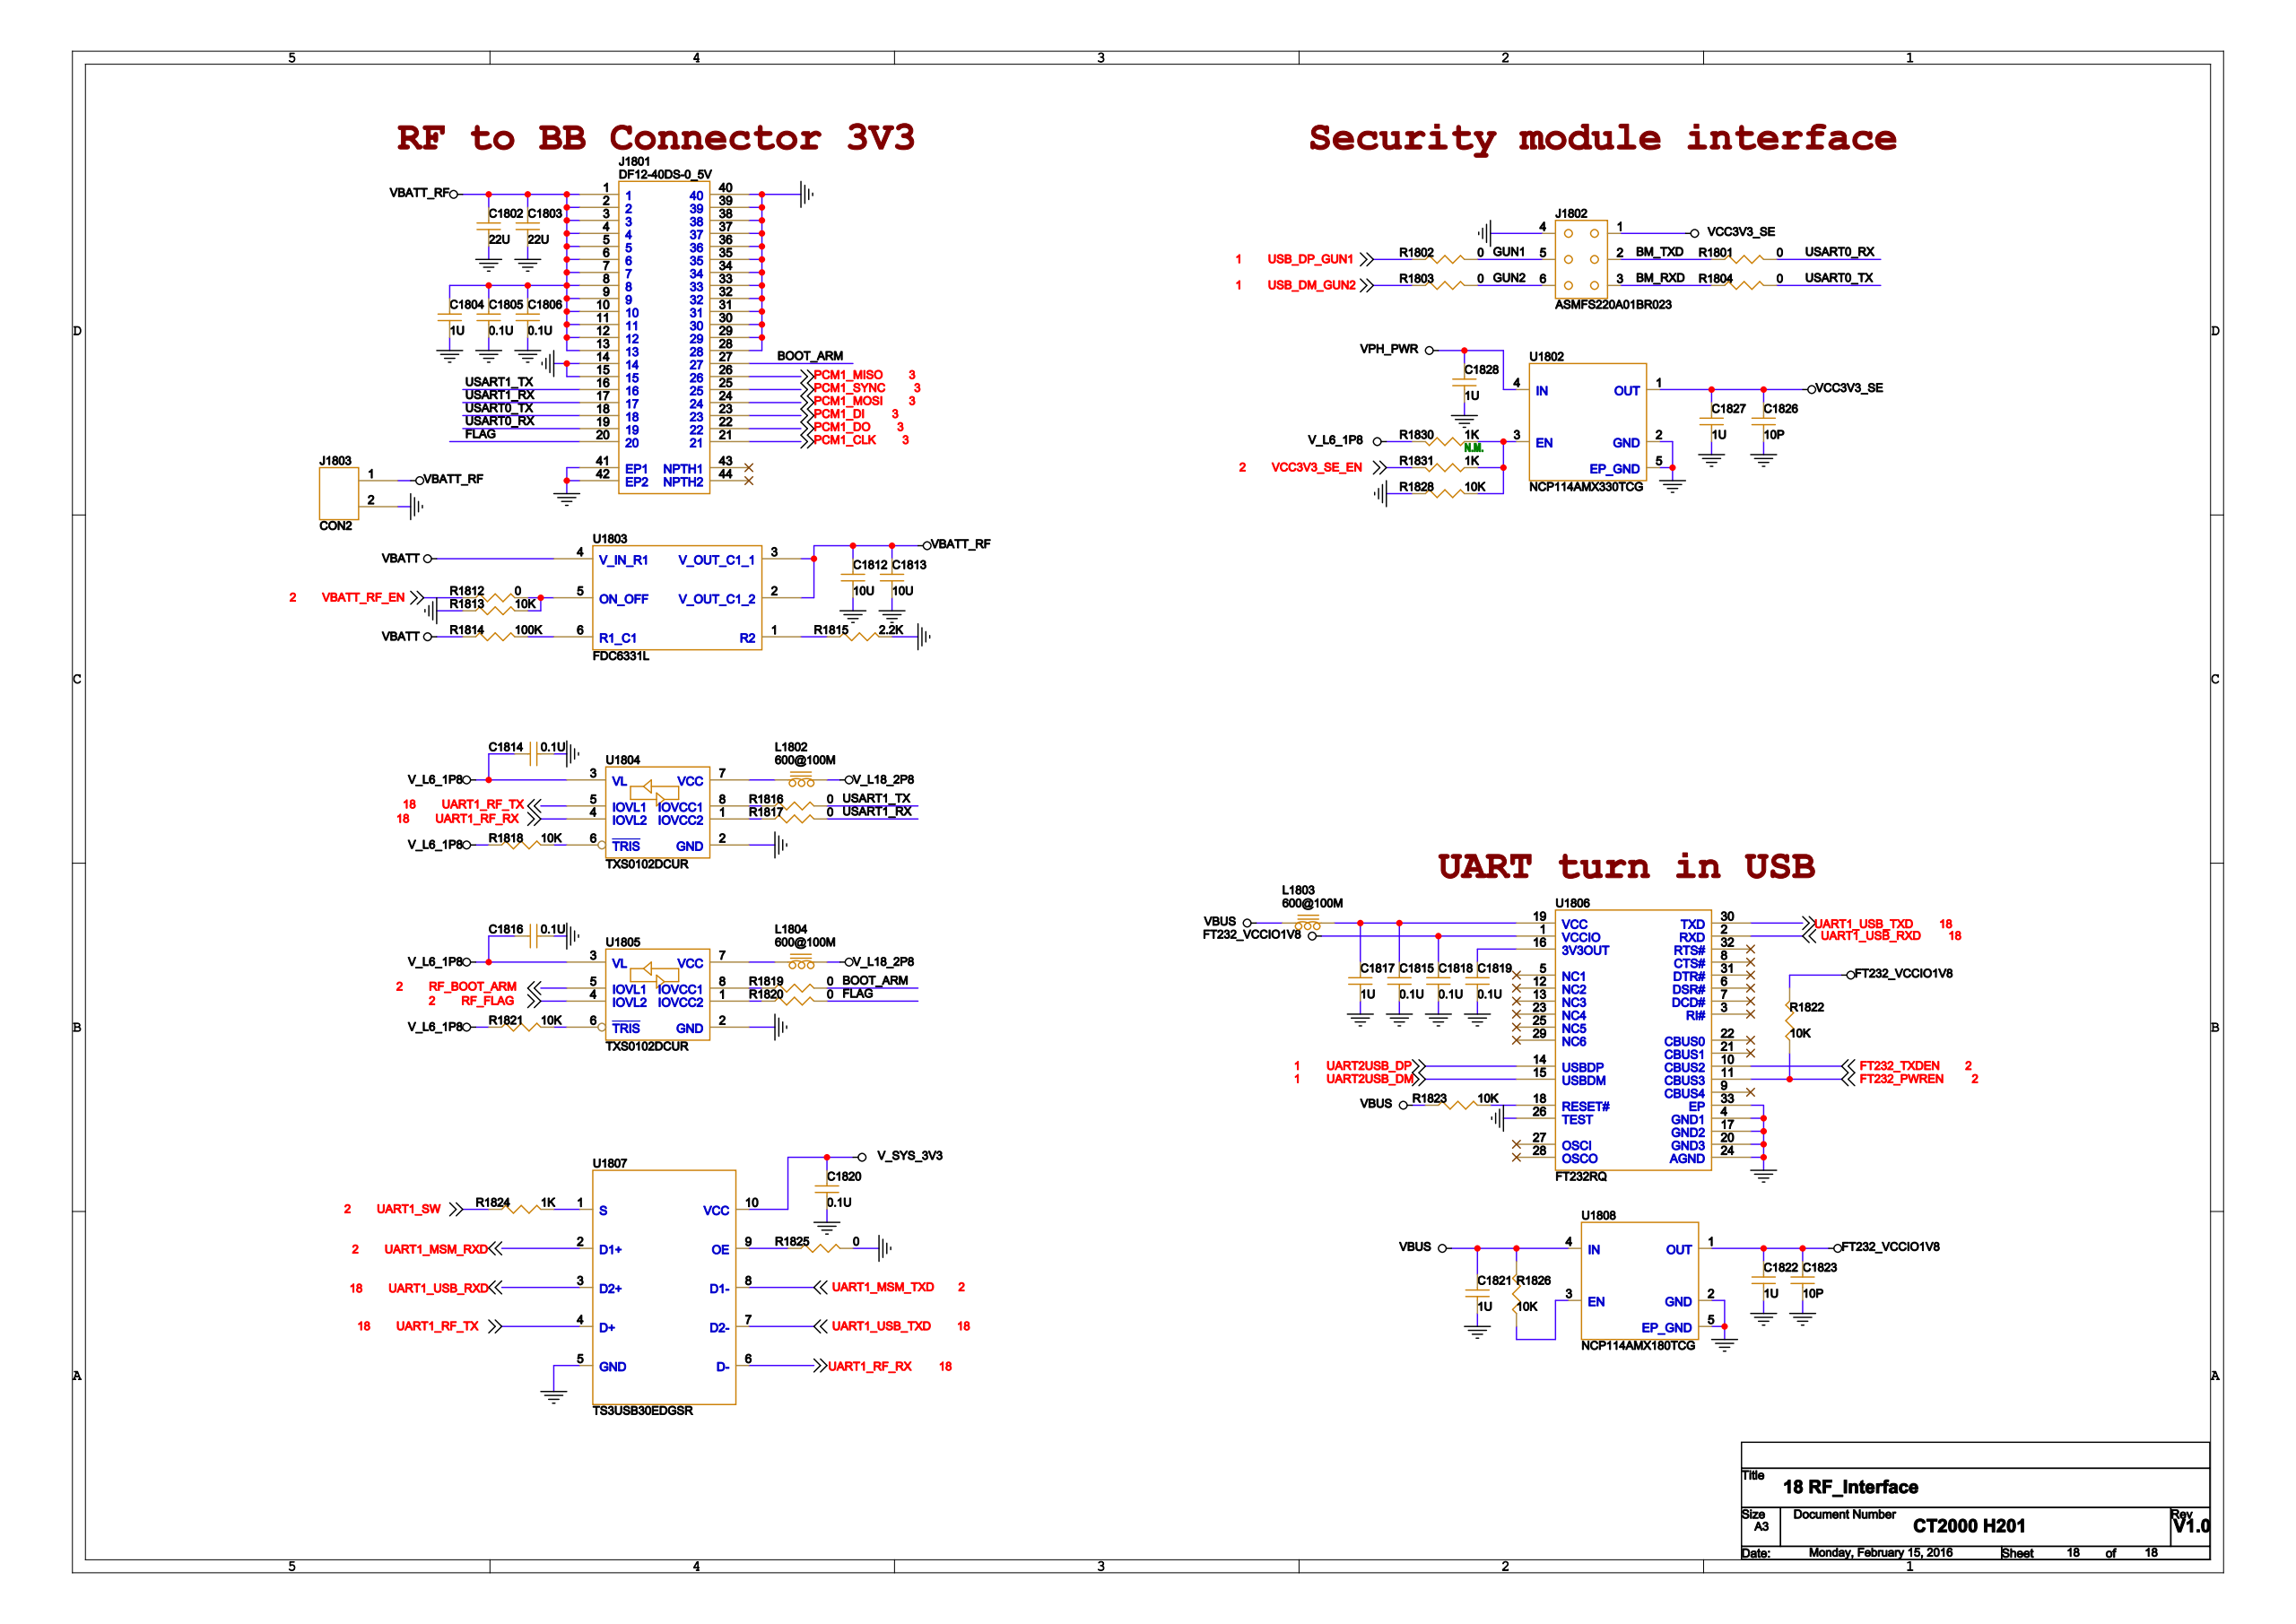Circuit board | Cadence Allegro | 573 parts | 376 nets | one sheet of the schematic
Parts on this sheet (reference | value | footprint):
C1802 | 22U | C0805
C1803 | 22U | C0805
C1804 | 1U | C0402
C1805 | 0.1U | C0402
C1806 | 0.1U | C0402
C1812 | 10U | C0603
C1813 | 10U | C0603
C1814 | 0.1U | C0402
C1815 | 0.1U | C0402
C1816 | 0.1U | C0402
C1817 | 1U | C0402
C1818 | 0.1U | C0402
C1819 | 0.1U | C0402
C1820 | 0.1U | C0402
C1821 | 1U | C0402
C1822 | 1U | C0402
C1823 | 10P | C0402
C1826 | 10P | C0402
C1827 | 1U | C0402
C1828 | 1U | C0402
J1801 | DF12-40DS-0_5V | BTB_DF12-40DS-0_5V_CCW
J1802 | ASMFS220A01BR023 | CON6_ASMFS220A01BR023
J1803 | CON2 | SIP2_2_54P
L1802 | 600@100M | L0402
L1803 | 600@100M | L0402
L1804 | 600@100M | L0402
R1801 | 0 | R0402
R1802 | 0 | R0402
R1803 | 0 | R0402
R1804 | 0 | R0402
R1812 | 0 | R0402
R1813 | 10K | R0402
R1814 | 100K | R0402
R1815 | 2.2K | R0402
R1816 | 0 | R0402
R1817 | 0 | R0402
R1818 | 10K | R0402
R1819 | 0 | R0402
R1820 | 0 | R0402
R1821 | 10K | R0402
R1822 | 10K | R0402
R1823 | 10K | R0402
R1824 | 1K | R0402
R1825 | 0 | R0402
R1826 | 10K | R0402
R1828 | 10K | R0402
R1830 | 1K | R0402
R1831 | 1K | R0402
U1802 | NCP114AMX330TCG | UDFN4_1X1X0P7_0P65
U1803 | FDC6331L | SSOT6_1P7X3
U1804 | TXS0102DCUR | SOT-70
U1805 | TXS0102DCUR | SOT-70
U1806 | FT232RQ | QFN32_5X5X0P9_0P5
U1807 | TS3USB30EDGSR | TS3USB30EDGSR
U1808 | NCP114AMX180TCG | UDFN4_1X1X0P7_0P65
Nets of these parts (net: part-pin ...):
GND: C1802-2 C1803-2 C1804-2 C1805-2 C1806-2 C1812-2 C1813-2 C1814-2 C1815-2 C1816-2 C1817-2 C1818-2 C1819-2 C1820-2 C1821-2 C1822-2 C1823-2 C1826-2 C1827-2 C1828-2 J1802-4 J1803-2 R1813-2 R1815-2 R1825-2 R1828-1 U1802-2 U1802-5 U1804-2 U1805-2 U1806-4 U1806-17 U1806-20 U1806-24 U1806-26 U1806-33 U1807-5 U1808-2 U1808-5 J1801-1 J1801-2 J1801-3 J1801-4 J1801-5 J1801-6 J1801-7 J1801-8 J1801-9 J1801-10 J1801-11 J1801-12 J1801-13 J1801-26 J1801-27 J1801-41 J1801-42
N52696315: C1819-1 U1806-16
FT232_TXDEN: U1806-10
FT232_PWREN: R1822-2 U1806-11
N52696194: R1823-1 U1806-18
UART1_USB_RXD: U1806-2 U1807-3
UART1_USB_TXD: U1806-30 U1807-7
UART2USB_DM: U1806-15
UART2USB_DP: U1806-14
N52698432: C1815-1 C1817-1 L1803-1 U1806-19
FT232_VCCIO1V8: C1818-1 C1822-1 C1823-1 R1822-1 U1806-1 U1808-1
V_SYS_3V3: C1820-1 U1807-10
VBATT: R1814-1 U1803-4
VPH_PWR: C1828-1 U1802-4
BOOT_ARM: R1819-2 J1801-14
PCM1_MISO: J1801-15
PCM1_SYNC: J1801-16
PCM1_MOSI: J1801-17
PCM1_DI: J1801-18
PCM1_DO: J1801-19
PCM1_CLK: J1801-20
FLAG: R1820-2 J1801-21
USART0_RX: R1801-2 J1801-22
USART0_TX: R1804-2 J1801-23
USART1_RX: R1817-2 J1801-24
USART1_TX: R1816-2 J1801-25
VBATT_RF: C1802-1 C1803-1 C1804-1 C1805-1 C1806-1 C1812-1 C1813-1 J1803-1 U1803-2 U1803-3 J1801-28 J1801-29 J1801-30 J1801-31 J1801-32 J1801-33 J1801-34 J1801-35 J1801-36 J1801-37 J1801-38 J1801-39 J1801-40
VCC3V3_SE: C1826-1 C1827-1 J1802-1 U1802-1
BM_TXD: J1802-2 R1801-1
BM_RXD: J1802-3 R1804-1
GUN1: J1802-5 R1802-2
GUN2: J1802-6 R1803-2
USB_DM_GUN2: R1803-1
USB_DP_GUN1: R1802-1
N52704005: R1826-2 U1808-3
VBUS: C1821-1 L1803-2 R1823-2 R1826-1 U1808-4
VBATT_RF_EN: R1812-1
UART1_MSM_RXD: U1807-2
UART1_MSM_TXD: U1807-8
V_L6_1P8: C1814-1 C1816-1 R1818-1 R1821-1 R1830-2 U1804-3 U1805-3
RF_BOOT_ARM: U1805-5
RF_FLAG: U1805-4
VCC3V3_SE_EN: R1831-2
UART1_SW: R1824-1
VCC3V3_RFIO: L1802-2 L1804-2
N52755623: L1802-1 U1804-7
N52758844: L1804-1 U1805-7
N52856260: R1828-2 R1830-1 R1831-1 U1802-3
N52674574: R1812-2 R1813-1 U1803-5
N52755629: R1818-2 U1804-6
N52758850: R1821-2 U1805-6
N52757691: R1816-1 U1804-8
N52755610: R1817-1 U1804-1
N52758889: R1819-1 U1805-8
N52758830: R1820-1 U1805-1
N52583772: R1825-1 U1807-9
N52583706: R1824-2 U1807-1
N52674540: R1815-1 U1803-1
N52674566: R1814-2 U1803-6
UART1_RF_TX: U1804-5 U1807-4
UART1_RF_RX: U1804-4 U1807-6